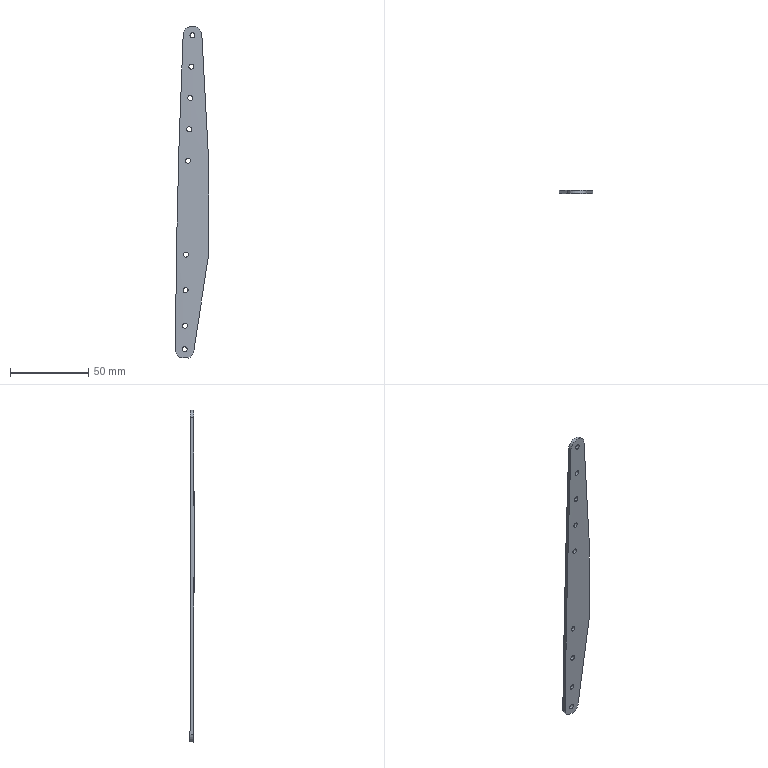Part | SolidWorks | features BaseBody 1 | 1 solid | 28 faces | box 21.224 x 2.686 x 212 mm | volume 6961 mm3 | cylinder 21 | plane 4 | spline 3 | commonest cylinder face diameters 3.2 x18 12 x3